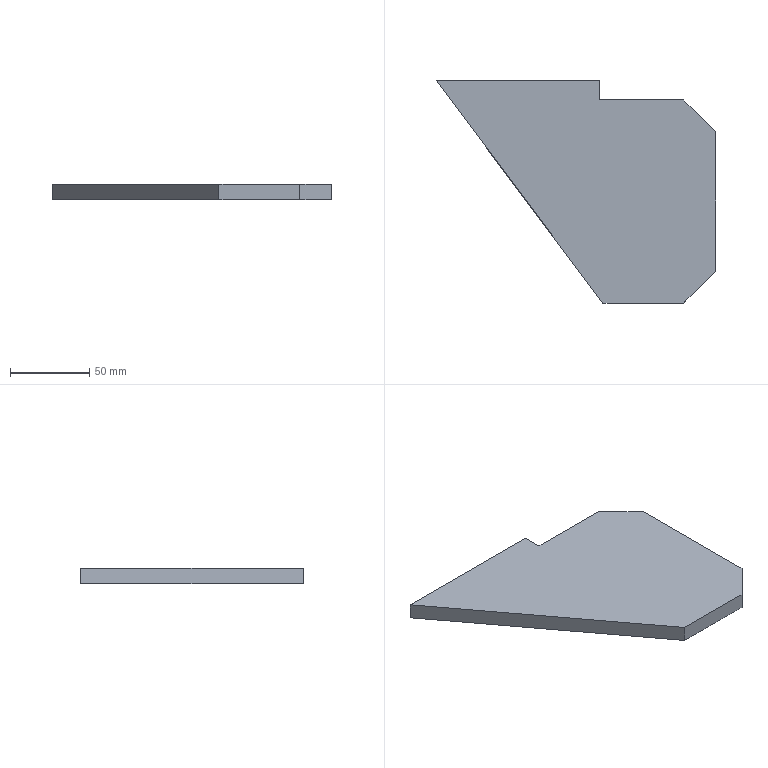Part | STEP file | 05 Rib plate | 1 solid | 10 faces | box 176 x 140 x 10 mm | volume 160140 mm3 | plane 10
STEP:
#1=CARTESIAN_POINT('',(0.,0.,0.));
#2=DIRECTION('',(0.,0.,1.));
#3=DIRECTION('',(1.,0.,0.));
#4=AXIS2_PLACEMENT_3D('',#1,#2,#3);
#5=CARTESIAN_POINT('',(0.,0.,0.));
#6=VERTEX_POINT('',#5);
#7=CARTESIAN_POINT('',(105.,-140.,0.));
#8=VERTEX_POINT('',#7);
#9=CARTESIAN_POINT('',(0.,0.,0.));
#10=DIRECTION('',(0.6,-0.8,0.));
#11=VECTOR('',#10,1.);
#12=LINE('',#9,#11);
#13=CARTESIAN_POINT('',(0.,0.,10.));
#14=DIRECTION('',(0.8,0.6,0.));
#15=DIRECTION('',(-0.6,0.8,0.));
#16=AXIS2_PLACEMENT_3D('',#13,#14,#15);
#17=PLANE('',#16);
#18=CARTESIAN_POINT('',(0.,-10.));
#19=DIRECTION('',(-1.,0.));
#20=VECTOR('',#19,1.);
#21=LINE('',#18,#20);
#22=(GEOMETRIC_REPRESENTATION_CONTEXT(2)PARAMETRIC_REPRESENTATION_CONTEXT()REPRESENTATION_CONTEXT('',''));
#23=DEFINITIONAL_REPRESENTATION('',(#21),#22);
#24=PCURVE('',#17,#23);
#25=CARTESIAN_POINT('',(0.,0.,0.));
#26=DIRECTION('',(0.,0.,1.));
#27=DIRECTION('',(1.,0.,0.));
#28=AXIS2_PLACEMENT_3D('',#25,#26,#27);
#29=PLANE('',#28);
#30=CARTESIAN_POINT('',(0.,0.));
#31=DIRECTION('',(0.6,-0.8));
#32=VECTOR('',#31,1.);
#33=LINE('',#30,#32);
#34=(GEOMETRIC_REPRESENTATION_CONTEXT(2)PARAMETRIC_REPRESENTATION_CONTEXT()REPRESENTATION_CONTEXT('',''));
#35=DEFINITIONAL_REPRESENTATION('',(#33),#34);
#36=PCURVE('',#29,#35);
#37=SURFACE_CURVE('',#12,(#24,#36),.PCURVE_S1.);
#38=EDGE_CURVE('',#6,#8,#37,.T.);
#39=ORIENTED_EDGE('',*,*,#38,.T.);
#40=CARTESIAN_POINT('',(105.,-140.,10.));
#41=VERTEX_POINT('',#40);
#42=CARTESIAN_POINT('',(105.,-140.,10.));
#43=DIRECTION('',(0.,0.,-1.));
#44=VECTOR('',#43,1.);
#45=LINE('',#42,#44);
#46=CARTESIAN_POINT('',(-175.,0.));
#47=DIRECTION('',(0.,-1.));
#48=VECTOR('',#47,1.);
#49=LINE('',#46,#48);
#50=(GEOMETRIC_REPRESENTATION_CONTEXT(2)PARAMETRIC_REPRESENTATION_CONTEXT()REPRESENTATION_CONTEXT('',''));
#51=DEFINITIONAL_REPRESENTATION('',(#49),#50);
#52=PCURVE('',#17,#51);
#53=CARTESIAN_POINT('',(105.,-140.,10.));
#54=DIRECTION('',(0.,1.,0.));
#55=DIRECTION('',(0.,0.,1.));
#56=AXIS2_PLACEMENT_3D('',#53,#54,#55);
#57=PLANE('',#56);
#58=CARTESIAN_POINT('',(0.,0.));
#59=DIRECTION('',(-1.,0.));
#60=VECTOR('',#59,1.);
#61=LINE('',#58,#60);
#62=(GEOMETRIC_REPRESENTATION_CONTEXT(2)PARAMETRIC_REPRESENTATION_CONTEXT()REPRESENTATION_CONTEXT('',''));
#63=DEFINITIONAL_REPRESENTATION('',(#61),#62);
#64=PCURVE('',#57,#63);
#65=SURFACE_CURVE('',#45,(#52,#64),.PCURVE_S1.);
#66=EDGE_CURVE('',#41,#8,#65,.T.);
#67=ORIENTED_EDGE('',*,*,#66,.F.);
#68=CARTESIAN_POINT('',(0.,0.,10.));
#69=VERTEX_POINT('',#68);
#70=CARTESIAN_POINT('',(0.,0.,10.));
#71=DIRECTION('',(0.6,-0.8,0.));
#72=VECTOR('',#71,1.);
#73=LINE('',#70,#72);
#74=CARTESIAN_POINT('',(0.,0.));
#75=DIRECTION('',(-1.,0.));
#76=VECTOR('',#75,1.);
#77=LINE('',#74,#76);
#78=(GEOMETRIC_REPRESENTATION_CONTEXT(2)PARAMETRIC_REPRESENTATION_CONTEXT()REPRESENTATION_CONTEXT('',''));
#79=DEFINITIONAL_REPRESENTATION('',(#77),#78);
#80=PCURVE('',#17,#79);
#81=CARTESIAN_POINT('',(0.,0.,10.));
#82=DIRECTION('',(0.,0.,1.));
#83=DIRECTION('',(1.,0.,0.));
#84=AXIS2_PLACEMENT_3D('',#81,#82,#83);
#85=PLANE('',#84);
#86=CARTESIAN_POINT('',(0.,0.));
#87=DIRECTION('',(0.6,-0.8));
#88=VECTOR('',#87,1.);
#89=LINE('',#86,#88);
#90=(GEOMETRIC_REPRESENTATION_CONTEXT(2)PARAMETRIC_REPRESENTATION_CONTEXT()REPRESENTATION_CONTEXT('',''));
#91=DEFINITIONAL_REPRESENTATION('',(#89),#90);
#92=PCURVE('',#85,#91);
#93=SURFACE_CURVE('',#73,(#80,#92),.PCURVE_S1.);
#94=EDGE_CURVE('',#69,#41,#93,.T.);
#95=ORIENTED_EDGE('',*,*,#94,.F.);
#96=CARTESIAN_POINT('',(0.,0.,10.));
#97=DIRECTION('',(0.,0.,-1.));
#98=VECTOR('',#97,1.);
#99=LINE('',#96,#98);
#100=CARTESIAN_POINT('',(0.,0.));
#101=DIRECTION('',(0.,-1.));
#102=VECTOR('',#101,1.);
#103=LINE('',#100,#102);
#104=(GEOMETRIC_REPRESENTATION_CONTEXT(2)PARAMETRIC_REPRESENTATION_CONTEXT()REPRESENTATION_CONTEXT('',''));
#105=DEFINITIONAL_REPRESENTATION('',(#103),#104);
#106=PCURVE('',#17,#105);
#107=CARTESIAN_POINT('',(0.,0.,10.));
#108=DIRECTION('',(0.,-1.,0.));
#109=DIRECTION('',(0.,0.,-1.));
#110=AXIS2_PLACEMENT_3D('',#107,#108,#109);
#111=PLANE('',#110);
#112=CARTESIAN_POINT('',(0.,0.));
#113=DIRECTION('',(1.,0.));
#114=VECTOR('',#113,1.);
#115=LINE('',#112,#114);
#116=(GEOMETRIC_REPRESENTATION_CONTEXT(2)PARAMETRIC_REPRESENTATION_CONTEXT()REPRESENTATION_CONTEXT('',''));
#117=DEFINITIONAL_REPRESENTATION('',(#115),#116);
#118=PCURVE('',#111,#117);
#119=SURFACE_CURVE('',#99,(#106,#118),.PCURVE_S1.);
#120=EDGE_CURVE('',#69,#6,#119,.T.);
#121=ORIENTED_EDGE('',*,*,#120,.T.);
#122=EDGE_LOOP('',(#39,#67,#95,#121));
#123=FACE_BOUND('',#122,.T.);
#124=ADVANCED_FACE('',(#123),#17,.F.);
#125=CARTESIAN_POINT('',(156.,-140.,0.));
#126=VERTEX_POINT('',#125);
#127=CARTESIAN_POINT('',(105.,-140.,0.));
#128=DIRECTION('',(1.,0.,0.));
#129=VECTOR('',#128,1.);
#130=LINE('',#127,#129);
#131=CARTESIAN_POINT('',(-10.,0.));
#132=DIRECTION('',(0.,1.));
#133=VECTOR('',#132,1.);
#134=LINE('',#131,#133);
#135=(GEOMETRIC_REPRESENTATION_CONTEXT(2)PARAMETRIC_REPRESENTATION_CONTEXT()REPRESENTATION_CONTEXT('',''));
#136=DEFINITIONAL_REPRESENTATION('',(#134),#135);
#137=PCURVE('',#57,#136);
#138=CARTESIAN_POINT('',(105.,-140.));
#139=DIRECTION('',(1.,0.));
#140=VECTOR('',#139,1.);
#141=LINE('',#138,#140);
#142=(GEOMETRIC_REPRESENTATION_CONTEXT(2)PARAMETRIC_REPRESENTATION_CONTEXT()REPRESENTATION_CONTEXT('',''));
#143=DEFINITIONAL_REPRESENTATION('',(#141),#142);
#144=PCURVE('',#29,#143);
#145=SURFACE_CURVE('',#130,(#137,#144),.PCURVE_S1.);
#146=EDGE_CURVE('',#8,#126,#145,.T.);
#147=ORIENTED_EDGE('',*,*,#146,.T.);
#148=CARTESIAN_POINT('',(156.,-140.,10.));
#149=VERTEX_POINT('',#148);
#150=CARTESIAN_POINT('',(156.,-140.,10.));
#151=DIRECTION('',(0.,0.,-1.));
#152=VECTOR('',#151,1.);
#153=LINE('',#150,#152);
#154=CARTESIAN_POINT('',(0.,51.));
#155=DIRECTION('',(-1.,0.));
#156=VECTOR('',#155,1.);
#157=LINE('',#154,#156);
#158=(GEOMETRIC_REPRESENTATION_CONTEXT(2)PARAMETRIC_REPRESENTATION_CONTEXT()REPRESENTATION_CONTEXT('',''));
#159=DEFINITIONAL_REPRESENTATION('',(#157),#158);
#160=PCURVE('',#57,#159);
#161=CARTESIAN_POINT('',(156.,-140.,10.));
#162=DIRECTION('',(-0.7071,0.7071,0.));
#163=DIRECTION('',(-0.7071,-0.7071,0.));
#164=AXIS2_PLACEMENT_3D('',#161,#162,#163);
#165=PLANE('',#164);
#166=CARTESIAN_POINT('',(0.,0.));
#167=DIRECTION('',(0.,-1.));
#168=VECTOR('',#167,1.);
#169=LINE('',#166,#168);
#170=(GEOMETRIC_REPRESENTATION_CONTEXT(2)PARAMETRIC_REPRESENTATION_CONTEXT()REPRESENTATION_CONTEXT('',''));
#171=DEFINITIONAL_REPRESENTATION('',(#169),#170);
#172=PCURVE('',#165,#171);
#173=SURFACE_CURVE('',#153,(#160,#172),.PCURVE_S1.);
#174=EDGE_CURVE('',#149,#126,#173,.T.);
#175=ORIENTED_EDGE('',*,*,#174,.F.);
#176=CARTESIAN_POINT('',(105.,-140.,10.));
#177=DIRECTION('',(1.,0.,0.));
#178=VECTOR('',#177,1.);
#179=LINE('',#176,#178);
#180=CARTESIAN_POINT('',(0.,0.));
#181=DIRECTION('',(0.,1.));
#182=VECTOR('',#181,1.);
#183=LINE('',#180,#182);
#184=(GEOMETRIC_REPRESENTATION_CONTEXT(2)PARAMETRIC_REPRESENTATION_CONTEXT()REPRESENTATION_CONTEXT('',''));
#185=DEFINITIONAL_REPRESENTATION('',(#183),#184);
#186=PCURVE('',#57,#185);
#187=CARTESIAN_POINT('',(105.,-140.));
#188=DIRECTION('',(1.,0.));
#189=VECTOR('',#188,1.);
#190=LINE('',#187,#189);
#191=(GEOMETRIC_REPRESENTATION_CONTEXT(2)PARAMETRIC_REPRESENTATION_CONTEXT()REPRESENTATION_CONTEXT('',''));
#192=DEFINITIONAL_REPRESENTATION('',(#190),#191);
#193=PCURVE('',#85,#192);
#194=SURFACE_CURVE('',#179,(#186,#193),.PCURVE_S1.);
#195=EDGE_CURVE('',#41,#149,#194,.T.);
#196=ORIENTED_EDGE('',*,*,#195,.F.);
#197=ORIENTED_EDGE('',*,*,#66,.T.);
#198=EDGE_LOOP('',(#147,#175,#196,#197));
#199=FACE_BOUND('',#198,.T.);
#200=ADVANCED_FACE('',(#199),#57,.F.);
#201=CARTESIAN_POINT('',(176.,-120.,0.));
#202=VERTEX_POINT('',#201);
#203=CARTESIAN_POINT('',(156.,-140.,0.));
#204=DIRECTION('',(0.7071,0.7071,0.));
#205=VECTOR('',#204,1.);
#206=LINE('',#203,#205);
#207=CARTESIAN_POINT('',(0.,-10.));
#208=DIRECTION('',(-1.,0.));
#209=VECTOR('',#208,1.);
#210=LINE('',#207,#209);
#211=(GEOMETRIC_REPRESENTATION_CONTEXT(2)PARAMETRIC_REPRESENTATION_CONTEXT()REPRESENTATION_CONTEXT('',''));
#212=DEFINITIONAL_REPRESENTATION('',(#210),#211);
#213=PCURVE('',#165,#212);
#214=CARTESIAN_POINT('',(156.,-140.));
#215=DIRECTION('',(0.7071,0.7071));
#216=VECTOR('',#215,1.);
#217=LINE('',#214,#216);
#218=(GEOMETRIC_REPRESENTATION_CONTEXT(2)PARAMETRIC_REPRESENTATION_CONTEXT()REPRESENTATION_CONTEXT('',''));
#219=DEFINITIONAL_REPRESENTATION('',(#217),#218);
#220=PCURVE('',#29,#219);
#221=SURFACE_CURVE('',#206,(#213,#220),.PCURVE_S1.);
#222=EDGE_CURVE('',#126,#202,#221,.T.);
#223=ORIENTED_EDGE('',*,*,#222,.T.);
#224=CARTESIAN_POINT('',(176.,-120.,10.));
#225=VERTEX_POINT('',#224);
#226=CARTESIAN_POINT('',(176.,-120.,10.));
#227=DIRECTION('',(0.,0.,-1.));
#228=VECTOR('',#227,1.);
#229=LINE('',#226,#228);
#230=CARTESIAN_POINT('',(-28.284,0.));
#231=DIRECTION('',(0.,-1.));
#232=VECTOR('',#231,1.);
#233=LINE('',#230,#232);
#234=(GEOMETRIC_REPRESENTATION_CONTEXT(2)PARAMETRIC_REPRESENTATION_CONTEXT()REPRESENTATION_CONTEXT('',''));
#235=DEFINITIONAL_REPRESENTATION('',(#233),#234);
#236=PCURVE('',#165,#235);
#237=CARTESIAN_POINT('',(176.,-32.,10.));
#238=DIRECTION('',(-1.,0.,0.));
#239=DIRECTION('',(0.,-1.,0.));
#240=AXIS2_PLACEMENT_3D('',#237,#238,#239);
#241=PLANE('',#240);
#242=CARTESIAN_POINT('',(88.,0.));
#243=DIRECTION('',(0.,-1.));
#244=VECTOR('',#243,1.);
#245=LINE('',#242,#244);
#246=(GEOMETRIC_REPRESENTATION_CONTEXT(2)PARAMETRIC_REPRESENTATION_CONTEXT()REPRESENTATION_CONTEXT('',''));
#247=DEFINITIONAL_REPRESENTATION('',(#245),#246);
#248=PCURVE('',#241,#247);
#249=SURFACE_CURVE('',#229,(#236,#248),.PCURVE_S1.);
#250=EDGE_CURVE('',#225,#202,#249,.T.);
#251=ORIENTED_EDGE('',*,*,#250,.F.);
#252=CARTESIAN_POINT('',(156.,-140.,10.));
#253=DIRECTION('',(0.7071,0.7071,0.));
#254=VECTOR('',#253,1.);
#255=LINE('',#252,#254);
#256=CARTESIAN_POINT('',(0.,0.));
#257=DIRECTION('',(-1.,0.));
#258=VECTOR('',#257,1.);
#259=LINE('',#256,#258);
#260=(GEOMETRIC_REPRESENTATION_CONTEXT(2)PARAMETRIC_REPRESENTATION_CONTEXT()REPRESENTATION_CONTEXT('',''));
#261=DEFINITIONAL_REPRESENTATION('',(#259),#260);
#262=PCURVE('',#165,#261);
#263=CARTESIAN_POINT('',(156.,-140.));
#264=DIRECTION('',(0.7071,0.7071));
#265=VECTOR('',#264,1.);
#266=LINE('',#263,#265);
#267=(GEOMETRIC_REPRESENTATION_CONTEXT(2)PARAMETRIC_REPRESENTATION_CONTEXT()REPRESENTATION_CONTEXT('',''));
#268=DEFINITIONAL_REPRESENTATION('',(#266),#267);
#269=PCURVE('',#85,#268);
#270=SURFACE_CURVE('',#255,(#262,#269),.PCURVE_S1.);
#271=EDGE_CURVE('',#149,#225,#270,.T.);
#272=ORIENTED_EDGE('',*,*,#271,.F.);
#273=ORIENTED_EDGE('',*,*,#174,.T.);
#274=EDGE_LOOP('',(#223,#251,#272,#273));
#275=FACE_BOUND('',#274,.T.);
#276=ADVANCED_FACE('',(#275),#165,.F.);
#277=CARTESIAN_POINT('',(176.,-32.,0.));
#278=VERTEX_POINT('',#277);
#279=CARTESIAN_POINT('',(176.,-32.,0.));
#280=DIRECTION('',(0.,1.,0.));
#281=VECTOR('',#280,1.);
#282=LINE('',#279,#281);
#283=CARTESIAN_POINT('',(0.,-10.));
#284=DIRECTION('',(-1.,0.));
#285=VECTOR('',#284,1.);
#286=LINE('',#283,#285);
#287=(GEOMETRIC_REPRESENTATION_CONTEXT(2)PARAMETRIC_REPRESENTATION_CONTEXT()REPRESENTATION_CONTEXT('',''));
#288=DEFINITIONAL_REPRESENTATION('',(#286),#287);
#289=PCURVE('',#241,#288);
#290=CARTESIAN_POINT('',(176.,-32.));
#291=DIRECTION('',(0.,1.));
#292=VECTOR('',#291,1.);
#293=LINE('',#290,#292);
#294=(GEOMETRIC_REPRESENTATION_CONTEXT(2)PARAMETRIC_REPRESENTATION_CONTEXT()REPRESENTATION_CONTEXT('',''));
#295=DEFINITIONAL_REPRESENTATION('',(#293),#294);
#296=PCURVE('',#29,#295);
#297=SURFACE_CURVE('',#282,(#289,#296),.PCURVE_S1.);
#298=EDGE_CURVE('',#202,#278,#297,.T.);
#299=ORIENTED_EDGE('',*,*,#298,.T.);
#300=CARTESIAN_POINT('',(176.,-32.,10.));
#301=VERTEX_POINT('',#300);
#302=CARTESIAN_POINT('',(176.,-32.,10.));
#303=DIRECTION('',(0.,0.,-1.));
#304=VECTOR('',#303,1.);
#305=LINE('',#302,#304);
#306=CARTESIAN_POINT('',(0.,0.));
#307=DIRECTION('',(0.,-1.));
#308=VECTOR('',#307,1.);
#309=LINE('',#306,#308);
#310=(GEOMETRIC_REPRESENTATION_CONTEXT(2)PARAMETRIC_REPRESENTATION_CONTEXT()REPRESENTATION_CONTEXT('',''));
#311=DEFINITIONAL_REPRESENTATION('',(#309),#310);
#312=PCURVE('',#241,#311);
#313=CARTESIAN_POINT('',(156.,-12.,10.));
#314=DIRECTION('',(-0.7071,-0.7071,0.));
#315=DIRECTION('',(0.7071,-0.7071,0.));
#316=AXIS2_PLACEMENT_3D('',#313,#314,#315);
#317=PLANE('',#316);
#318=CARTESIAN_POINT('',(28.284,0.));
#319=DIRECTION('',(0.,-1.));
#320=VECTOR('',#319,1.);
#321=LINE('',#318,#320);
#322=(GEOMETRIC_REPRESENTATION_CONTEXT(2)PARAMETRIC_REPRESENTATION_CONTEXT()REPRESENTATION_CONTEXT('',''));
#323=DEFINITIONAL_REPRESENTATION('',(#321),#322);
#324=PCURVE('',#317,#323);
#325=SURFACE_CURVE('',#305,(#312,#324),.PCURVE_S1.);
#326=EDGE_CURVE('',#301,#278,#325,.T.);
#327=ORIENTED_EDGE('',*,*,#326,.F.);
#328=CARTESIAN_POINT('',(176.,-32.,10.));
#329=DIRECTION('',(0.,1.,0.));
#330=VECTOR('',#329,1.);
#331=LINE('',#328,#330);
#332=CARTESIAN_POINT('',(0.,0.));
#333=DIRECTION('',(-1.,0.));
#334=VECTOR('',#333,1.);
#335=LINE('',#332,#334);
#336=(GEOMETRIC_REPRESENTATION_CONTEXT(2)PARAMETRIC_REPRESENTATION_CONTEXT()REPRESENTATION_CONTEXT('',''));
#337=DEFINITIONAL_REPRESENTATION('',(#335),#336);
#338=PCURVE('',#241,#337);
#339=CARTESIAN_POINT('',(176.,-32.));
#340=DIRECTION('',(0.,1.));
#341=VECTOR('',#340,1.);
#342=LINE('',#339,#341);
#343=(GEOMETRIC_REPRESENTATION_CONTEXT(2)PARAMETRIC_REPRESENTATION_CONTEXT()REPRESENTATION_CONTEXT('',''));
#344=DEFINITIONAL_REPRESENTATION('',(#342),#343);
#345=PCURVE('',#85,#344);
#346=SURFACE_CURVE('',#331,(#338,#345),.PCURVE_S1.);
#347=EDGE_CURVE('',#225,#301,#346,.T.);
#348=ORIENTED_EDGE('',*,*,#347,.F.);
#349=ORIENTED_EDGE('',*,*,#250,.T.);
#350=EDGE_LOOP('',(#299,#327,#348,#349));
#351=FACE_BOUND('',#350,.T.);
#352=ADVANCED_FACE('',(#351),#241,.F.);
#353=CARTESIAN_POINT('',(156.,-12.,0.));
#354=VERTEX_POINT('',#353);
#355=CARTESIAN_POINT('',(156.,-12.,0.));
#356=DIRECTION('',(-0.7071,0.7071,0.));
#357=VECTOR('',#356,1.);
#358=LINE('',#355,#357);
#359=CARTESIAN_POINT('',(0.,-10.));
#360=DIRECTION('',(-1.,0.));
#361=VECTOR('',#360,1.);
#362=LINE('',#359,#361);
#363=(GEOMETRIC_REPRESENTATION_CONTEXT(2)PARAMETRIC_REPRESENTATION_CONTEXT()REPRESENTATION_CONTEXT('',''));
#364=DEFINITIONAL_REPRESENTATION('',(#362),#363);
#365=PCURVE('',#317,#364);
#366=CARTESIAN_POINT('',(156.,-12.));
#367=DIRECTION('',(-0.7071,0.7071));
#368=VECTOR('',#367,1.);
#369=LINE('',#366,#368);
#370=(GEOMETRIC_REPRESENTATION_CONTEXT(2)PARAMETRIC_REPRESENTATION_CONTEXT()REPRESENTATION_CONTEXT('',''));
#371=DEFINITIONAL_REPRESENTATION('',(#369),#370);
#372=PCURVE('',#29,#371);
#373=SURFACE_CURVE('',#358,(#365,#372),.PCURVE_S1.);
#374=EDGE_CURVE('',#278,#354,#373,.T.);
#375=ORIENTED_EDGE('',*,*,#374,.T.);
#376=CARTESIAN_POINT('',(156.,-12.,10.));
#377=VERTEX_POINT('',#376);
#378=CARTESIAN_POINT('',(156.,-12.,10.));
#379=DIRECTION('',(0.,0.,-1.));
#380=VECTOR('',#379,1.);
#381=LINE('',#378,#380);
#382=CARTESIAN_POINT('',(0.,0.));
#383=DIRECTION('',(0.,-1.));
#384=VECTOR('',#383,1.);
#385=LINE('',#382,#384);
#386=(GEOMETRIC_REPRESENTATION_CONTEXT(2)PARAMETRIC_REPRESENTATION_CONTEXT()REPRESENTATION_CONTEXT('',''));
#387=DEFINITIONAL_REPRESENTATION('',(#385),#386);
#388=PCURVE('',#317,#387);
#389=CARTESIAN_POINT('',(103.,-12.,10.));
#390=DIRECTION('',(0.,-1.,0.));
#391=DIRECTION('',(0.,0.,-1.));
#392=AXIS2_PLACEMENT_3D('',#389,#390,#391);
#393=PLANE('',#392);
#394=CARTESIAN_POINT('',(0.,53.));
#395=DIRECTION('',(1.,0.));
#396=VECTOR('',#395,1.);
#397=LINE('',#394,#396);
#398=(GEOMETRIC_REPRESENTATION_CONTEXT(2)PARAMETRIC_REPRESENTATION_CONTEXT()REPRESENTATION_CONTEXT('',''));
#399=DEFINITIONAL_REPRESENTATION('',(#397),#398);
#400=PCURVE('',#393,#399);
#401=SURFACE_CURVE('',#381,(#388,#400),.PCURVE_S1.);
#402=EDGE_CURVE('',#377,#354,#401,.T.);
#403=ORIENTED_EDGE('',*,*,#402,.F.);
#404=CARTESIAN_POINT('',(156.,-12.,10.));
#405=DIRECTION('',(-0.7071,0.7071,0.));
#406=VECTOR('',#405,1.);
#407=LINE('',#404,#406);
#408=CARTESIAN_POINT('',(0.,0.));
#409=DIRECTION('',(-1.,0.));
#410=VECTOR('',#409,1.);
#411=LINE('',#408,#410);
#412=(GEOMETRIC_REPRESENTATION_CONTEXT(2)PARAMETRIC_REPRESENTATION_CONTEXT()REPRESENTATION_CONTEXT('',''));
#413=DEFINITIONAL_REPRESENTATION('',(#411),#412);
#414=PCURVE('',#317,#413);
#415=CARTESIAN_POINT('',(156.,-12.));
#416=DIRECTION('',(-0.7071,0.7071));
#417=VECTOR('',#416,1.);
#418=LINE('',#415,#417);
#419=(GEOMETRIC_REPRESENTATION_CONTEXT(2)PARAMETRIC_REPRESENTATION_CONTEXT()REPRESENTATION_CONTEXT('',''));
#420=DEFINITIONAL_REPRESENTATION('',(#418),#419);
#421=PCURVE('',#85,#420);
#422=SURFACE_CURVE('',#407,(#414,#421),.PCURVE_S1.);
#423=EDGE_CURVE('',#301,#377,#422,.T.);
#424=ORIENTED_EDGE('',*,*,#423,.F.);
#425=ORIENTED_EDGE('',*,*,#326,.T.);
#426=EDGE_LOOP('',(#375,#403,#424,#425));
#427=FACE_BOUND('',#426,.T.);
#428=ADVANCED_FACE('',(#427),#317,.F.);
#429=CARTESIAN_POINT('',(103.,-12.,0.));
#430=VERTEX_POINT('',#429);
#431=CARTESIAN_POINT('',(103.,-12.,0.));
#432=DIRECTION('',(-1.,0.,0.));
#433=VECTOR('',#432,1.);
#434=LINE('',#431,#433);
#435=CARTESIAN_POINT('',(10.,0.));
#436=DIRECTION('',(0.,-1.));
#437=VECTOR('',#436,1.);
#438=LINE('',#435,#437);
#439=(GEOMETRIC_REPRESENTATION_CONTEXT(2)PARAMETRIC_REPRESENTATION_CONTEXT()REPRESENTATION_CONTEXT('',''));
#440=DEFINITIONAL_REPRESENTATION('',(#438),#439);
#441=PCURVE('',#393,#440);
#442=CARTESIAN_POINT('',(103.,-12.));
#443=DIRECTION('',(-1.,0.));
#444=VECTOR('',#443,1.);
#445=LINE('',#442,#444);
#446=(GEOMETRIC_REPRESENTATION_CONTEXT(2)PARAMETRIC_REPRESENTATION_CONTEXT()REPRESENTATION_CONTEXT('',''));
#447=DEFINITIONAL_REPRESENTATION('',(#445),#446);
#448=PCURVE('',#29,#447);
#449=SURFACE_CURVE('',#434,(#441,#448),.PCURVE_S1.);
#450=EDGE_CURVE('',#354,#430,#449,.T.);
#451=ORIENTED_EDGE('',*,*,#450,.T.);
#452=CARTESIAN_POINT('',(103.,-12.,10.));
#453=VERTEX_POINT('',#452);
#454=CARTESIAN_POINT('',(103.,-12.,10.));
#455=DIRECTION('',(0.,0.,-1.));
#456=VECTOR('',#455,1.);
#457=LINE('',#454,#456);
#458=CARTESIAN_POINT('',(0.,0.));
#459=DIRECTION('',(1.,0.));
#460=VECTOR('',#459,1.);
#461=LINE('',#458,#460);
#462=(GEOMETRIC_REPRESENTATION_CONTEXT(2)PARAMETRIC_REPRESENTATION_CONTEXT()REPRESENTATION_CONTEXT('',''));
#463=DEFINITIONAL_REPRESENTATION('',(#461),#462);
#464=PCURVE('',#393,#463);
#465=CARTESIAN_POINT('',(103.,0.,10.));
#466=DIRECTION('',(-1.,0.,0.));
#467=DIRECTION('',(0.,0.,1.));
#468=AXIS2_PLACEMENT_3D('',#465,#466,#467);
#469=PLANE('',#468);
#470=CARTESIAN_POINT('',(0.,-12.));
#471=DIRECTION('',(-1.,0.));
#472=VECTOR('',#471,1.);
#473=LINE('',#470,#472);
#474=(GEOMETRIC_REPRESENTATION_CONTEXT(2)PARAMETRIC_REPRESENTATION_CONTEXT()REPRESENTATION_CONTEXT('',''));
#475=DEFINITIONAL_REPRESENTATION('',(#473),#474);
#476=PCURVE('',#469,#475);
#477=SURFACE_CURVE('',#457,(#464,#476),.PCURVE_S1.);
#478=EDGE_CURVE('',#453,#430,#477,.T.);
#479=ORIENTED_EDGE('',*,*,#478,.F.);
#480=CARTESIAN_POINT('',(103.,-12.,10.));
#481=DIRECTION('',(-1.,0.,0.));
#482=VECTOR('',#481,1.);
#483=LINE('',#480,#482);
#484=CARTESIAN_POINT('',(0.,0.));
#485=DIRECTION('',(0.,-1.));
#486=VECTOR('',#485,1.);
#487=LINE('',#484,#486);
#488=(GEOMETRIC_REPRESENTATION_CONTEXT(2)PARAMETRIC_REPRESENTATION_CONTEXT()REPRESENTATION_CONTEXT('',''));
#489=DEFINITIONAL_REPRESENTATION('',(#487),#488);
#490=PCURVE('',#393,#489);
#491=CARTESIAN_POINT('',(103.,-12.));
#492=DIRECTION('',(-1.,0.));
#493=VECTOR('',#492,1.);
#494=LINE('',#491,#493);
#495=(GEOMETRIC_REPRESENTATION_CONTEXT(2)PARAMETRIC_REPRESENTATION_CONTEXT()REPRESENTATION_CONTEXT('',''));
#496=DEFINITIONAL_REPRESENTATION('',(#494),#495);
#497=PCURVE('',#85,#496);
#498=SURFACE_CURVE('',#483,(#490,#497),.PCURVE_S1.);
#499=EDGE_CURVE('',#377,#453,#498,.T.);
#500=ORIENTED_EDGE('',*,*,#499,.F.);
#501=ORIENTED_EDGE('',*,*,#402,.T.);
#502=EDGE_LOOP('',(#451,#479,#500,#501));
#503=FACE_BOUND('',#502,.T.);
#504=ADVANCED_FACE('',(#503),#393,.F.);
#505=CARTESIAN_POINT('',(103.,0.,0.));
#506=VERTEX_POINT('',#505);
#507=CARTESIAN_POINT('',(103.,0.,0.));
#508=DIRECTION('',(0.,1.,0.));
#509=VECTOR('',#508,1.);
#510=LINE('',#507,#509);
#511=CARTESIAN_POINT('',(-10.,0.));
#512=DIRECTION('',(0.,1.));
#513=VECTOR('',#512,1.);
#514=LINE('',#511,#513);
#515=(GEOMETRIC_REPRESENTATION_CONTEXT(2)PARAMETRIC_REPRESENTATION_CONTEXT()REPRESENTATION_CONTEXT('',''));
#516=DEFINITIONAL_REPRESENTATION('',(#514),#515);
#517=PCURVE('',#469,#516);
#518=CARTESIAN_POINT('',(103.,0.));
#519=DIRECTION('',(0.,1.));
#520=VECTOR('',#519,1.);
#521=LINE('',#518,#520);
#522=(GEOMETRIC_REPRESENTATION_CONTEXT(2)PARAMETRIC_REPRESENTATION_CONTEXT()REPRESENTATION_CONTEXT('',''));
#523=DEFINITIONAL_REPRESENTATION('',(#521),#522);
#524=PCURVE('',#29,#523);
#525=SURFACE_CURVE('',#510,(#517,#524),.PCURVE_S1.);
#526=EDGE_CURVE('',#430,#506,#525,.T.);
#527=ORIENTED_EDGE('',*,*,#526,.T.);
#528=CARTESIAN_POINT('',(103.,0.,10.));
#529=VERTEX_POINT('',#528);
#530=CARTESIAN_POINT('',(103.,0.,10.));
#531=DIRECTION('',(0.,0.,-1.));
#532=VECTOR('',#531,1.);
#533=LINE('',#530,#532);
#534=CARTESIAN_POINT('',(0.,0.));
#535=DIRECTION('',(-1.,0.));
#536=VECTOR('',#535,1.);
#537=LINE('',#534,#536);
#538=(GEOMETRIC_REPRESENTATION_CONTEXT(2)PARAMETRIC_REPRESENTATION_CONTEXT()REPRESENTATION_CONTEXT('',''));
#539=DEFINITIONAL_REPRESENTATION('',(#537),#538);
#540=PCURVE('',#469,#539);
#541=CARTESIAN_POINT('',(0.,103.));
#542=DIRECTION('',(1.,0.));
#543=VECTOR('',#542,1.);
#544=LINE('',#541,#543);
#545=(GEOMETRIC_REPRESENTATION_CONTEXT(2)PARAMETRIC_REPRESENTATION_CONTEXT()REPRESENTATION_CONTEXT('',''));
#546=DEFINITIONAL_REPRESENTATION('',(#544),#545);
#547=PCURVE('',#111,#546);
#548=SURFACE_CURVE('',#533,(#540,#547),.PCURVE_S1.);
#549=EDGE_CURVE('',#529,#506,#548,.T.);
#550=ORIENTED_EDGE('',*,*,#549,.F.);
#551=CARTESIAN_POINT('',(103.,0.,10.));
#552=DIRECTION('',(0.,1.,0.));
#553=VECTOR('',#552,1.);
#554=LINE('',#551,#553);
#555=CARTESIAN_POINT('',(0.,0.));
#556=DIRECTION('',(0.,1.));
#557=VECTOR('',#556,1.);
#558=LINE('',#555,#557);
#559=(GEOMETRIC_REPRESENTATION_CONTEXT(2)PARAMETRIC_REPRESENTATION_CONTEXT()REPRESENTATION_CONTEXT('',''));
#560=DEFINITIONAL_REPRESENTATION('',(#558),#559);
#561=PCURVE('',#469,#560);
#562=CARTESIAN_POINT('',(103.,0.));
#563=DIRECTION('',(0.,1.));
#564=VECTOR('',#563,1.);
#565=LINE('',#562,#564);
#566=(GEOMETRIC_REPRESENTATION_CONTEXT(2)PARAMETRIC_REPRESENTATION_CONTEXT()REPRESENTATION_CONTEXT('',''));
#567=DEFINITIONAL_REPRESENTATION('',(#565),#566);
#568=PCURVE('',#85,#567);
#569=SURFACE_CURVE('',#554,(#561,#568),.PCURVE_S1.);
#570=EDGE_CURVE('',#453,#529,#569,.T.);
#571=ORIENTED_EDGE('',*,*,#570,.F.);
#572=ORIENTED_EDGE('',*,*,#478,.T.);
#573=EDGE_LOOP('',(#527,#550,#571,#572));
#574=FACE_BOUND('',#573,.T.);
#575=ADVANCED_FACE('',(#574),#469,.F.);
#576=CARTESIAN_POINT('',(0.,0.,0.));
#577=DIRECTION('',(-1.,0.,0.));
#578=VECTOR('',#577,1.);
#579=LINE('',#576,#578);
#580=CARTESIAN_POINT('',(10.,0.));
#581=DIRECTION('',(0.,-1.));
#582=VECTOR('',#581,1.);
#583=LINE('',#580,#582);
#584=(GEOMETRIC_REPRESENTATION_CONTEXT(2)PARAMETRIC_REPRESENTATION_CONTEXT()REPRESENTATION_CONTEXT('',''));
#585=DEFINITIONAL_REPRESENTATION('',(#583),#584);
#586=PCURVE('',#111,#585);
#587=CARTESIAN_POINT('',(0.,0.));
#588=DIRECTION('',(-1.,0.));
#589=VECTOR('',#588,1.);
#590=LINE('',#587,#589);
#591=(GEOMETRIC_REPRESENTATION_CONTEXT(2)PARAMETRIC_REPRESENTATION_CONTEXT()REPRESENTATION_CONTEXT('',''));
#592=DEFINITIONAL_REPRESENTATION('',(#590),#591);
#593=PCURVE('',#29,#592);
#594=SURFACE_CURVE('',#579,(#586,#593),.PCURVE_S1.);
#595=EDGE_CURVE('',#506,#6,#594,.T.);
#596=ORIENTED_EDGE('',*,*,#595,.T.);
#597=ORIENTED_EDGE('',*,*,#120,.F.);
#598=CARTESIAN_POINT('',(0.,0.,10.));
#599=DIRECTION('',(-1.,0.,0.));
#600=VECTOR('',#599,1.);
#601=LINE('',#598,#600);
#602=CARTESIAN_POINT('',(0.,0.));
#603=DIRECTION('',(0.,-1.));
#604=VECTOR('',#603,1.);
#605=LINE('',#602,#604);
#606=(GEOMETRIC_REPRESENTATION_CONTEXT(2)PARAMETRIC_REPRESENTATION_CONTEXT()REPRESENTATION_CONTEXT('',''));
#607=DEFINITIONAL_REPRESENTATION('',(#605),#606);
#608=PCURVE('',#111,#607);
#609=CARTESIAN_POINT('',(0.,0.));
#610=DIRECTION('',(-1.,0.));
#611=VECTOR('',#610,1.);
#612=LINE('',#609,#611);
#613=(GEOMETRIC_REPRESENTATION_CONTEXT(2)PARAMETRIC_REPRESENTATION_CONTEXT()REPRESENTATION_CONTEXT('',''));
#614=DEFINITIONAL_REPRESENTATION('',(#612),#613);
#615=PCURVE('',#85,#614);
#616=SURFACE_CURVE('',#601,(#608,#615),.PCURVE_S1.);
#617=EDGE_CURVE('',#529,#69,#616,.T.);
#618=ORIENTED_EDGE('',*,*,#617,.F.);
#619=ORIENTED_EDGE('',*,*,#549,.T.);
#620=EDGE_LOOP('',(#596,#597,#618,#619));
#621=FACE_BOUND('',#620,.T.);
#622=ADVANCED_FACE('',(#621),#111,.F.);
#623=ORIENTED_EDGE('',*,*,#94,.T.);
#624=ORIENTED_EDGE('',*,*,#195,.T.);
#625=ORIENTED_EDGE('',*,*,#271,.T.);
#626=ORIENTED_EDGE('',*,*,#347,.T.);
#627=ORIENTED_EDGE('',*,*,#423,.T.);
#628=ORIENTED_EDGE('',*,*,#499,.T.);
#629=ORIENTED_EDGE('',*,*,#570,.T.);
#630=ORIENTED_EDGE('',*,*,#617,.T.);
#631=EDGE_LOOP('',(#623,#624,#625,#626,#627,#628,#629,#630));
#632=FACE_BOUND('',#631,.T.);
#633=ADVANCED_FACE('',(#632),#85,.T.);
#634=ORIENTED_EDGE('',*,*,#38,.F.);
#635=ORIENTED_EDGE('',*,*,#595,.F.);
#636=ORIENTED_EDGE('',*,*,#526,.F.);
#637=ORIENTED_EDGE('',*,*,#450,.F.);
#638=ORIENTED_EDGE('',*,*,#374,.F.);
#639=ORIENTED_EDGE('',*,*,#298,.F.);
#640=ORIENTED_EDGE('',*,*,#222,.F.);
#641=ORIENTED_EDGE('',*,*,#146,.F.);
#642=EDGE_LOOP('',(#634,#635,#636,#637,#638,#639,#640,#641));
#643=FACE_BOUND('',#642,.T.);
#644=ADVANCED_FACE('',(#643),#29,.F.);
#645=CLOSED_SHELL('',(#124,#200,#276,#352,#428,#504,#575,#622,#633,#644));
#646=MANIFOLD_SOLID_BREP('',#645);
#647=(LENGTH_UNIT()NAMED_UNIT(*)SI_UNIT(.MILLI.,.METRE.));
#648=UNCERTAINTY_MEASURE_WITH_UNIT(LENGTH_MEASURE(0.0000001),#647,'','');
#649=(NAMED_UNIT(*)PLANE_ANGLE_UNIT()SI_UNIT($,.RADIAN.));
#650=(NAMED_UNIT(*)SI_UNIT($,.STERADIAN.)SOLID_ANGLE_UNIT());
#651=(GEOMETRIC_REPRESENTATION_CONTEXT(3)GLOBAL_UNCERTAINTY_ASSIGNED_CONTEXT((#648))GLOBAL_UNIT_ASSIGNED_CONTEXT((#647,#649,#650))REPRESENTATION_CONTEXT('',''));
#652=ADVANCED_BREP_SHAPE_REPRESENTATION('',(#4,#646),#651);